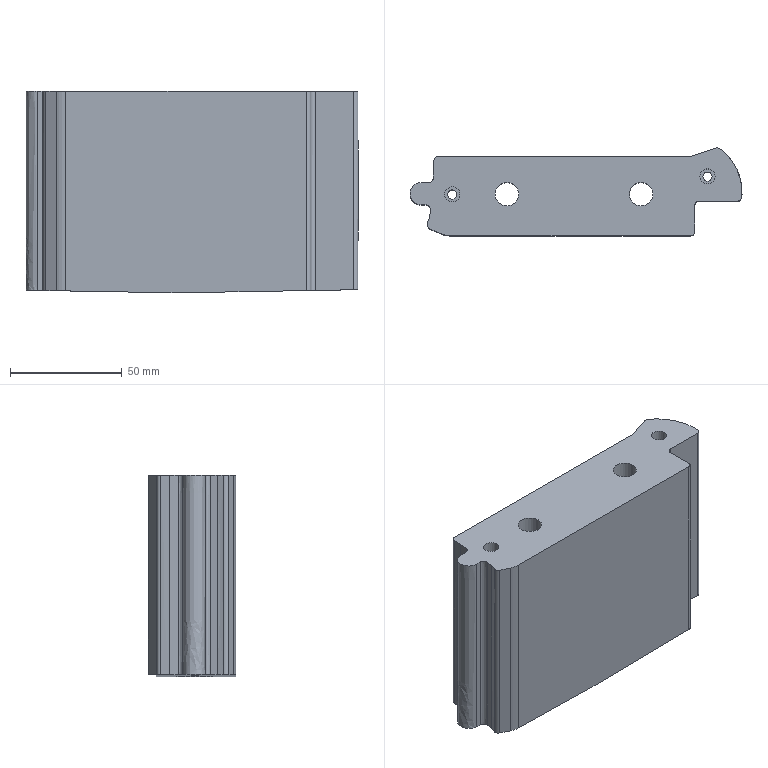Part | STEP file | gslz 2016.10.28-10_id2878_x_t | 1 solid | 41 faces | box 148.369 x 39.226 x 90 mm | volume 378722 mm3 | cylinder 15 | plane 13 | other 12 | spline 1 | commonest cylinder face diameters 4 x6 4.1 x2 6.8 x2 10.5 x2 17 x2 20 x1